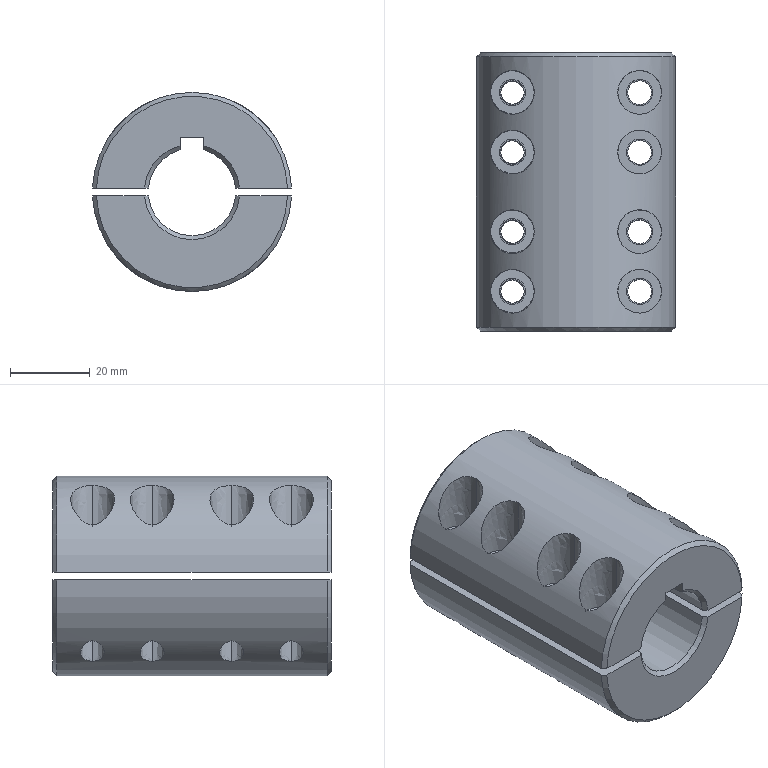Part | STEP file | COUPLING.stp | 2 solids | 82 faces | box 50.056 x 70 x 50.096 mm | volume 91173 mm3 | cylinder 29 | spline 28 | plane 15 | cone 10 | commonest cylinder face diameters 6 x8 6.6 x8 11 x8 22 x3 50.096 x2